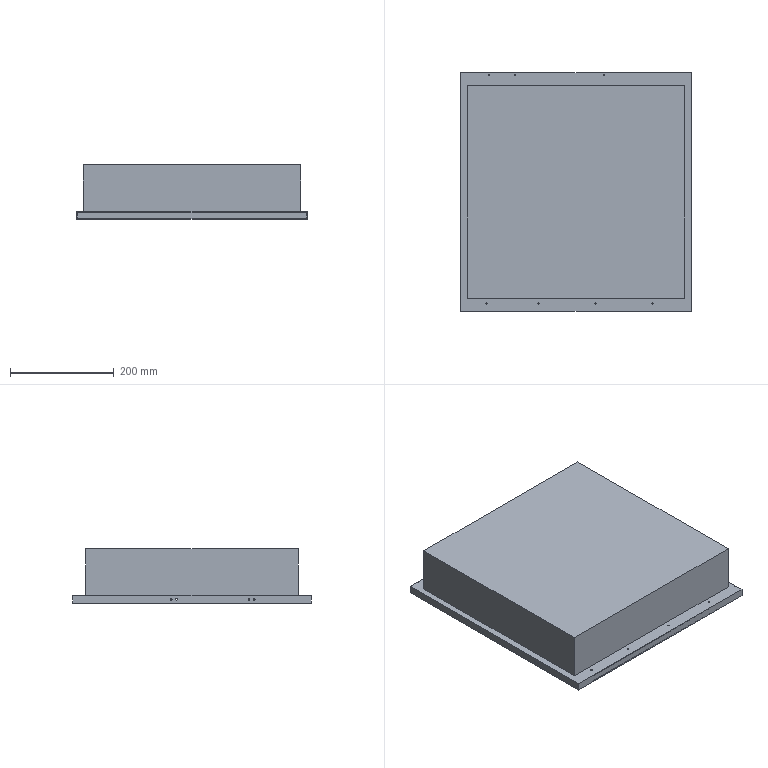Part | SolidWorks | features ICE 9, HoleWzd 5, MoveFace 2, Extrusion 1, Fillet 1, LPattern 1, Shell 1 | 1 solid | 165 faces | box 445 x 460 x 105 mm | volume 15966667 mm3 | cylinder 106 | plane 59 | commonest cylinder face diameters 2.5 x90 3.3 x16